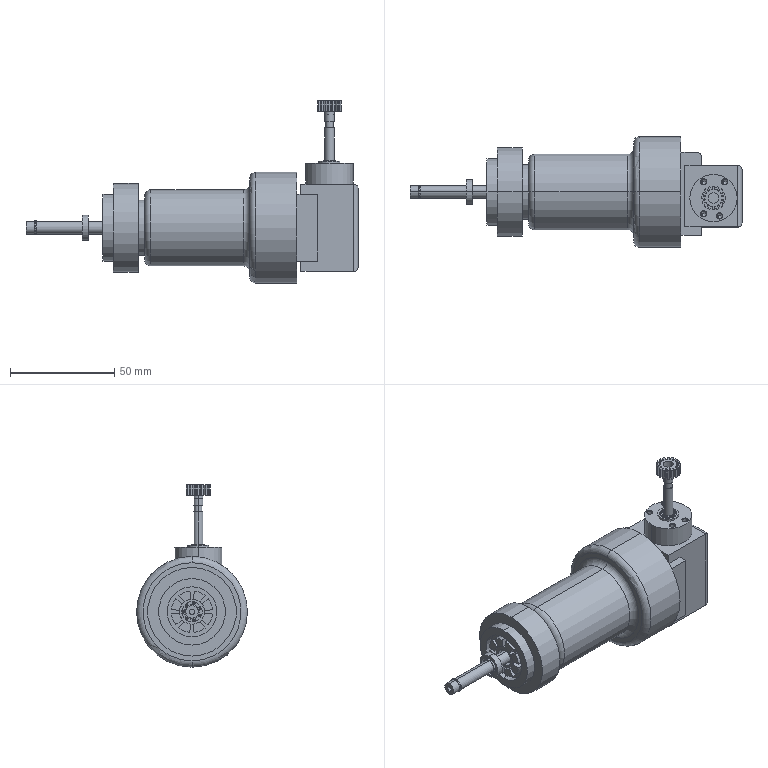Part | SolidWorks | features ICE 20, Fillet 3, HoleWzd 2, CirPattern 1, Revolution 1 | 2 solids | 365 faces | box 159.542 x 53.214 x 87.607 mm | volume 170177 mm3 | cylinder 192 | plane 133 | cone 30 | torus 10 | commonest cylinder face diameters 1.196 x49 1 x32 4.963 x16 0.95 x14 2.5 x10 12 x8